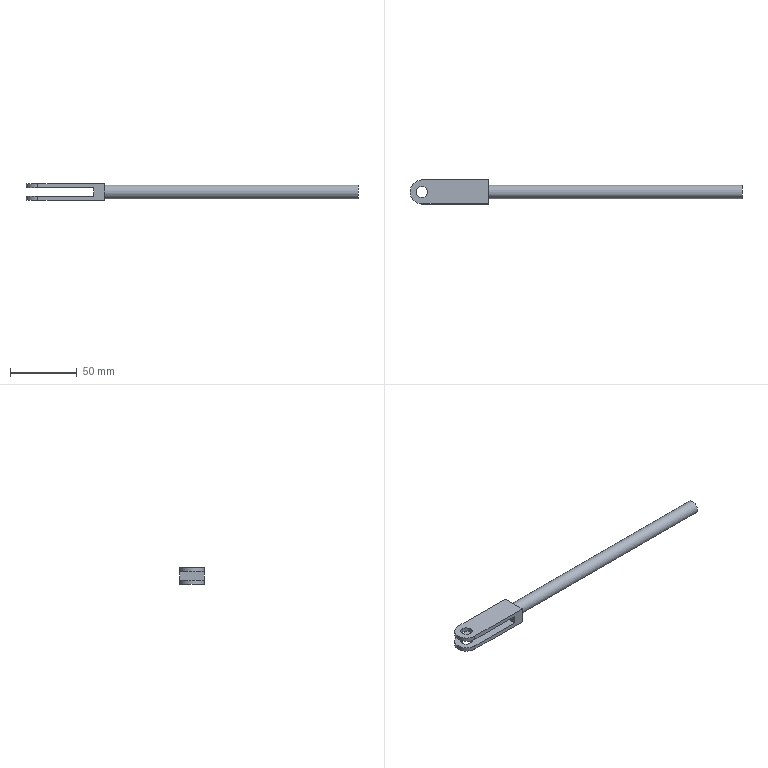Part | NX | features EXTRUDE 3, DATUM_CSYS 2, SKETCH 1, SWP104 1, UNITE 1 | 1 solid | 14 faces | box 249 x 18 x 12 mm | volume 21761 mm3 | plane 9 | cylinder 5 | commonest cylinder face diameters 8.5 x2 18 x2 10.051 x1
STEP:
#1=CARTESIAN_POINT('',(240.,0.,5.025));
#2=VERTEX_POINT('',#1);
#3=CARTESIAN_POINT('',(240.,0.,0.));
#4=DIRECTION('',(-1.,0.,0.));
#5=DIRECTION('',(0.,0.,1.));
#6=AXIS2_PLACEMENT_3D('',#3,#4,#5);
#7=CIRCLE('',#6,5.025);
#8=EDGE_CURVE('',#2,#2,#7,.T.);
#9=ORIENTED_EDGE('',*,*,#8,.F.);
#10=EDGE_LOOP('',(#9));
#11=FACE_BOUND('',#10,.T.);
#12=CARTESIAN_POINT('',(240.,0.,0.));
#13=DIRECTION('',(-1.,0.,0.));
#14=DIRECTION('',(0.,0.,1.));
#15=AXIS2_PLACEMENT_3D('',#12,#13,#14);
#16=PLANE('',#15);
#17=ADVANCED_FACE('',(#11),#16,.F.);
#18=ORIENTED_EDGE('',*,*,#8,.T.);
#19=EDGE_LOOP('',(#18));
#20=FACE_BOUND('',#19,.T.);
#21=CARTESIAN_POINT('',(50.,0.,5.025));
#22=VERTEX_POINT('',#21);
#23=CARTESIAN_POINT('',(50.,0.,0.));
#24=DIRECTION('',(-1.,0.,0.));
#25=DIRECTION('',(0.,0.,1.));
#26=AXIS2_PLACEMENT_3D('',#23,#24,#25);
#27=CIRCLE('',#26,5.025);
#28=EDGE_CURVE('',#22,#22,#27,.T.);
#29=ORIENTED_EDGE('',*,*,#28,.F.);
#30=EDGE_LOOP('',(#29));
#31=FACE_BOUND('',#30,.T.);
#32=CARTESIAN_POINT('',(50.,0.,0.));
#33=DIRECTION('',(-1.,0.,0.));
#34=DIRECTION('',(0.,0.,1.));
#35=AXIS2_PLACEMENT_3D('',#32,#33,#34);
#36=CYLINDRICAL_SURFACE('',#35,5.025);
#37=ADVANCED_FACE('',(#20,#31),#36,.T.);
#38=CARTESIAN_POINT('',(0.,9.,3.));
#39=VERTEX_POINT('',#38);
#40=CARTESIAN_POINT('',(0.,9.,6.));
#41=VERTEX_POINT('',#40);
#42=CARTESIAN_POINT('',(0.,9.,-6.));
#43=DIRECTION('',(0.,0.,1.));
#44=VECTOR('',#43,1000.);
#45=LINE('',#42,#44);
#46=EDGE_CURVE('',#39,#41,#45,.T.);
#47=ORIENTED_EDGE('',*,*,#46,.F.);
#48=CARTESIAN_POINT('',(0.,-9.,3.));
#49=VERTEX_POINT('',#48);
#50=CARTESIAN_POINT('',(0.,0.,3.));
#51=DIRECTION('',(0.,0.,1.));
#52=DIRECTION('',(-1.,0.,0.));
#53=AXIS2_PLACEMENT_3D('',#50,#51,#52);
#54=CIRCLE('',#53,9.);
#55=EDGE_CURVE('',#39,#49,#54,.T.);
#56=ORIENTED_EDGE('',*,*,#55,.T.);
#57=CARTESIAN_POINT('',(0.,-9.,6.));
#58=VERTEX_POINT('',#57);
#59=CARTESIAN_POINT('',(0.,-9.,-6.));
#60=DIRECTION('',(0.,0.,1.));
#61=VECTOR('',#60,1000.);
#62=LINE('',#59,#61);
#63=EDGE_CURVE('',#49,#58,#62,.T.);
#64=ORIENTED_EDGE('',*,*,#63,.T.);
#65=CARTESIAN_POINT('',(0.,0.,6.));
#66=DIRECTION('',(0.,0.,1.));
#67=DIRECTION('',(-1.,0.,0.));
#68=AXIS2_PLACEMENT_3D('',#65,#66,#67);
#69=CIRCLE('',#68,9.);
#70=EDGE_CURVE('',#41,#58,#69,.T.);
#71=ORIENTED_EDGE('',*,*,#70,.F.);
#72=EDGE_LOOP('',(#47,#56,#64,#71));
#73=FACE_BOUND('',#72,.T.);
#74=CARTESIAN_POINT('',(0.,0.,-6.));
#75=DIRECTION('',(0.,0.,1.));
#76=DIRECTION('',(1.,0.,0.));
#77=AXIS2_PLACEMENT_3D('',#74,#75,#76);
#78=CYLINDRICAL_SURFACE('',#77,9.);
#79=ADVANCED_FACE('',(#73),#78,.T.);
#80=CARTESIAN_POINT('',(42.,9.,-3.));
#81=VERTEX_POINT('',#80);
#82=CARTESIAN_POINT('',(0.,9.,-3.));
#83=VERTEX_POINT('',#82);
#84=CARTESIAN_POINT('',(42.,9.,-3.));
#85=DIRECTION('',(-1.,0.,0.));
#86=VECTOR('',#85,1000.);
#87=LINE('',#84,#86);
#88=EDGE_CURVE('',#81,#83,#87,.T.);
#89=ORIENTED_EDGE('',*,*,#88,.F.);
#90=CARTESIAN_POINT('',(42.,9.,3.));
#91=VERTEX_POINT('',#90);
#92=CARTESIAN_POINT('',(42.,9.,3.));
#93=DIRECTION('',(0.,0.,-1.));
#94=VECTOR('',#93,1000.);
#95=LINE('',#92,#94);
#96=EDGE_CURVE('',#91,#81,#95,.T.);
#97=ORIENTED_EDGE('',*,*,#96,.F.);
#98=CARTESIAN_POINT('',(42.,9.,3.));
#99=DIRECTION('',(-1.,0.,0.));
#100=VECTOR('',#99,1000.);
#101=LINE('',#98,#100);
#102=EDGE_CURVE('',#91,#39,#101,.T.);
#103=ORIENTED_EDGE('',*,*,#102,.T.);
#104=ORIENTED_EDGE('',*,*,#46,.T.);
#105=CARTESIAN_POINT('',(50.,9.,6.));
#106=VERTEX_POINT('',#105);
#107=CARTESIAN_POINT('',(50.,9.,6.));
#108=DIRECTION('',(-1.,0.,0.));
#109=VECTOR('',#108,1000.);
#110=LINE('',#107,#109);
#111=EDGE_CURVE('',#106,#41,#110,.T.);
#112=ORIENTED_EDGE('',*,*,#111,.F.);
#113=CARTESIAN_POINT('',(50.,9.,-6.));
#114=VERTEX_POINT('',#113);
#115=CARTESIAN_POINT('',(50.,9.,-6.));
#116=DIRECTION('',(0.,0.,1.));
#117=VECTOR('',#116,1000.);
#118=LINE('',#115,#117);
#119=EDGE_CURVE('',#114,#106,#118,.T.);
#120=ORIENTED_EDGE('',*,*,#119,.F.);
#121=CARTESIAN_POINT('',(0.,9.,-6.));
#122=VERTEX_POINT('',#121);
#123=CARTESIAN_POINT('',(50.,9.,-6.));
#124=DIRECTION('',(-1.,0.,0.));
#125=VECTOR('',#124,1000.);
#126=LINE('',#123,#125);
#127=EDGE_CURVE('',#114,#122,#126,.T.);
#128=ORIENTED_EDGE('',*,*,#127,.T.);
#129=CARTESIAN_POINT('',(0.,9.,-6.));
#130=DIRECTION('',(0.,0.,1.));
#131=VECTOR('',#130,1000.);
#132=LINE('',#129,#131);
#133=EDGE_CURVE('',#122,#83,#132,.T.);
#134=ORIENTED_EDGE('',*,*,#133,.T.);
#135=EDGE_LOOP('',(#89,#97,#103,#104,#112,#120,#128,#134));
#136=FACE_BOUND('',#135,.T.);
#137=CARTESIAN_POINT('',(50.,9.,-6.));
#138=DIRECTION('',(0.,1.,0.));
#139=DIRECTION('',(0.,0.,1.));
#140=AXIS2_PLACEMENT_3D('',#137,#138,#139);
#141=PLANE('',#140);
#142=ADVANCED_FACE('',(#136),#141,.T.);
#143=CARTESIAN_POINT('',(0.,-9.,-3.));
#144=VERTEX_POINT('',#143);
#145=CARTESIAN_POINT('',(0.,0.,-3.));
#146=DIRECTION('',(0.,0.,1.));
#147=DIRECTION('',(0.,1.,0.));
#148=AXIS2_PLACEMENT_3D('',#145,#146,#147);
#149=CIRCLE('',#148,9.);
#150=EDGE_CURVE('',#83,#144,#149,.T.);
#151=ORIENTED_EDGE('',*,*,#150,.F.);
#152=ORIENTED_EDGE('',*,*,#133,.F.);
#153=CARTESIAN_POINT('',(0.,-9.,-6.));
#154=VERTEX_POINT('',#153);
#155=CARTESIAN_POINT('',(0.,0.,-6.));
#156=DIRECTION('',(0.,0.,1.));
#157=DIRECTION('',(0.,1.,0.));
#158=AXIS2_PLACEMENT_3D('',#155,#156,#157);
#159=CIRCLE('',#158,9.);
#160=EDGE_CURVE('',#122,#154,#159,.T.);
#161=ORIENTED_EDGE('',*,*,#160,.T.);
#162=CARTESIAN_POINT('',(0.,-9.,-6.));
#163=DIRECTION('',(0.,0.,1.));
#164=VECTOR('',#163,1000.);
#165=LINE('',#162,#164);
#166=EDGE_CURVE('',#154,#144,#165,.T.);
#167=ORIENTED_EDGE('',*,*,#166,.T.);
#168=EDGE_LOOP('',(#151,#152,#161,#167));
#169=FACE_BOUND('',#168,.T.);
#170=CARTESIAN_POINT('',(0.,0.,-6.));
#171=DIRECTION('',(0.,0.,1.));
#172=DIRECTION('',(1.,0.,0.));
#173=AXIS2_PLACEMENT_3D('',#170,#171,#172);
#174=CYLINDRICAL_SURFACE('',#173,9.);
#175=ADVANCED_FACE('',(#169),#174,.T.);
#176=CARTESIAN_POINT('',(42.,-9.,-3.));
#177=VERTEX_POINT('',#176);
#178=CARTESIAN_POINT('',(0.,-9.,-3.));
#179=DIRECTION('',(1.,0.,0.));
#180=VECTOR('',#179,1000.);
#181=LINE('',#178,#180);
#182=EDGE_CURVE('',#144,#177,#181,.T.);
#183=ORIENTED_EDGE('',*,*,#182,.F.);
#184=ORIENTED_EDGE('',*,*,#166,.F.);
#185=CARTESIAN_POINT('',(50.,-9.,-6.));
#186=VERTEX_POINT('',#185);
#187=CARTESIAN_POINT('',(0.,-9.,-6.));
#188=DIRECTION('',(1.,0.,0.));
#189=VECTOR('',#188,1000.);
#190=LINE('',#187,#189);
#191=EDGE_CURVE('',#154,#186,#190,.T.);
#192=ORIENTED_EDGE('',*,*,#191,.T.);
#193=CARTESIAN_POINT('',(50.,-9.,6.));
#194=VERTEX_POINT('',#193);
#195=CARTESIAN_POINT('',(50.,-9.,-6.));
#196=DIRECTION('',(0.,0.,1.));
#197=VECTOR('',#196,1000.);
#198=LINE('',#195,#197);
#199=EDGE_CURVE('',#186,#194,#198,.T.);
#200=ORIENTED_EDGE('',*,*,#199,.T.);
#201=CARTESIAN_POINT('',(0.,-9.,6.));
#202=DIRECTION('',(1.,0.,0.));
#203=VECTOR('',#202,1000.);
#204=LINE('',#201,#203);
#205=EDGE_CURVE('',#58,#194,#204,.T.);
#206=ORIENTED_EDGE('',*,*,#205,.F.);
#207=ORIENTED_EDGE('',*,*,#63,.F.);
#208=CARTESIAN_POINT('',(42.,-9.,3.));
#209=VERTEX_POINT('',#208);
#210=CARTESIAN_POINT('',(0.,-9.,3.));
#211=DIRECTION('',(1.,0.,0.));
#212=VECTOR('',#211,1000.);
#213=LINE('',#210,#212);
#214=EDGE_CURVE('',#49,#209,#213,.T.);
#215=ORIENTED_EDGE('',*,*,#214,.T.);
#216=CARTESIAN_POINT('',(42.,-9.,3.));
#217=DIRECTION('',(0.,0.,-1.));
#218=VECTOR('',#217,1000.);
#219=LINE('',#216,#218);
#220=EDGE_CURVE('',#209,#177,#219,.T.);
#221=ORIENTED_EDGE('',*,*,#220,.T.);
#222=EDGE_LOOP('',(#183,#184,#192,#200,#206,#207,#215,#221));
#223=FACE_BOUND('',#222,.T.);
#224=CARTESIAN_POINT('',(0.,-9.,-6.));
#225=DIRECTION('',(0.,-1.,0.));
#226=DIRECTION('',(0.,0.,-1.));
#227=AXIS2_PLACEMENT_3D('',#224,#225,#226);
#228=PLANE('',#227);
#229=ADVANCED_FACE('',(#223),#228,.T.);
#230=ORIENTED_EDGE('',*,*,#28,.T.);
#231=EDGE_LOOP('',(#230));
#232=FACE_BOUND('',#231,.T.);
#233=CARTESIAN_POINT('',(50.,-9.,6.));
#234=DIRECTION('',(0.,1.,0.));
#235=VECTOR('',#234,1000.);
#236=LINE('',#233,#235);
#237=EDGE_CURVE('',#194,#106,#236,.T.);
#238=ORIENTED_EDGE('',*,*,#237,.F.);
#239=ORIENTED_EDGE('',*,*,#199,.F.);
#240=CARTESIAN_POINT('',(50.,-9.,-6.));
#241=DIRECTION('',(0.,1.,0.));
#242=VECTOR('',#241,1000.);
#243=LINE('',#240,#242);
#244=EDGE_CURVE('',#186,#114,#243,.T.);
#245=ORIENTED_EDGE('',*,*,#244,.T.);
#246=ORIENTED_EDGE('',*,*,#119,.T.);
#247=EDGE_LOOP('',(#238,#239,#245,#246));
#248=FACE_BOUND('',#247,.T.);
#249=CARTESIAN_POINT('',(50.,-9.,-6.));
#250=DIRECTION('',(1.,0.,0.));
#251=DIRECTION('',(0.,0.,-1.));
#252=AXIS2_PLACEMENT_3D('',#249,#250,#251);
#253=PLANE('',#252);
#254=ADVANCED_FACE('',(#232,#248),#253,.T.);
#255=CARTESIAN_POINT('',(4.25,0.,-6.));
#256=VERTEX_POINT('',#255);
#257=CARTESIAN_POINT('',(0.,0.,-6.));
#258=DIRECTION('',(0.,0.,1.));
#259=DIRECTION('',(1.,0.,0.));
#260=AXIS2_PLACEMENT_3D('',#257,#258,#259);
#261=CIRCLE('',#260,4.25);
#262=EDGE_CURVE('',#256,#256,#261,.F.);
#263=ORIENTED_EDGE('',*,*,#262,.F.);
#264=EDGE_LOOP('',(#263));
#265=FACE_BOUND('',#264,.T.);
#266=ORIENTED_EDGE('',*,*,#127,.F.);
#267=ORIENTED_EDGE('',*,*,#244,.F.);
#268=ORIENTED_EDGE('',*,*,#191,.F.);
#269=ORIENTED_EDGE('',*,*,#160,.F.);
#270=EDGE_LOOP('',(#266,#267,#268,#269));
#271=FACE_BOUND('',#270,.T.);
#272=CARTESIAN_POINT('',(0.,0.,-6.));
#273=DIRECTION('',(0.,0.,1.));
#274=DIRECTION('',(1.,0.,0.));
#275=AXIS2_PLACEMENT_3D('',#272,#273,#274);
#276=PLANE('',#275);
#277=ADVANCED_FACE('',(#265,#271),#276,.F.);
#278=CARTESIAN_POINT('',(4.25,0.,6.));
#279=VERTEX_POINT('',#278);
#280=CARTESIAN_POINT('',(0.,0.,6.));
#281=DIRECTION('',(0.,0.,1.));
#282=DIRECTION('',(1.,0.,0.));
#283=AXIS2_PLACEMENT_3D('',#280,#281,#282);
#284=CIRCLE('',#283,4.25);
#285=EDGE_CURVE('',#279,#279,#284,.F.);
#286=ORIENTED_EDGE('',*,*,#285,.T.);
#287=EDGE_LOOP('',(#286));
#288=FACE_BOUND('',#287,.T.);
#289=ORIENTED_EDGE('',*,*,#111,.T.);
#290=ORIENTED_EDGE('',*,*,#70,.T.);
#291=ORIENTED_EDGE('',*,*,#205,.T.);
#292=ORIENTED_EDGE('',*,*,#237,.T.);
#293=EDGE_LOOP('',(#289,#290,#291,#292));
#294=FACE_BOUND('',#293,.T.);
#295=CARTESIAN_POINT('',(0.,0.,6.));
#296=DIRECTION('',(0.,0.,1.));
#297=DIRECTION('',(1.,0.,0.));
#298=AXIS2_PLACEMENT_3D('',#295,#296,#297);
#299=PLANE('',#298);
#300=ADVANCED_FACE('',(#288,#294),#299,.T.);
#301=CARTESIAN_POINT('',(42.,-9.,-3.));
#302=DIRECTION('',(0.,1.,0.));
#303=VECTOR('',#302,1000.);
#304=LINE('',#301,#303);
#305=EDGE_CURVE('',#81,#177,#304,.F.);
#306=ORIENTED_EDGE('',*,*,#305,.T.);
#307=ORIENTED_EDGE('',*,*,#220,.F.);
#308=CARTESIAN_POINT('',(42.,-9.,3.));
#309=DIRECTION('',(0.,1.,0.));
#310=VECTOR('',#309,1000.);
#311=LINE('',#308,#310);
#312=EDGE_CURVE('',#91,#209,#311,.F.);
#313=ORIENTED_EDGE('',*,*,#312,.F.);
#314=ORIENTED_EDGE('',*,*,#96,.T.);
#315=EDGE_LOOP('',(#306,#307,#313,#314));
#316=FACE_BOUND('',#315,.T.);
#317=CARTESIAN_POINT('',(42.,-9.,3.));
#318=DIRECTION('',(-1.,0.,0.));
#319=DIRECTION('',(0.,0.,1.));
#320=AXIS2_PLACEMENT_3D('',#317,#318,#319);
#321=PLANE('',#320);
#322=ADVANCED_FACE('',(#316),#321,.T.);
#323=CARTESIAN_POINT('',(4.25,0.,3.));
#324=VERTEX_POINT('',#323);
#325=CARTESIAN_POINT('',(0.,0.,3.));
#326=DIRECTION('',(0.,0.,1.));
#327=DIRECTION('',(1.,0.,0.));
#328=AXIS2_PLACEMENT_3D('',#325,#326,#327);
#329=CIRCLE('',#328,4.25);
#330=EDGE_CURVE('',#324,#324,#329,.F.);
#331=ORIENTED_EDGE('',*,*,#330,.F.);
#332=EDGE_LOOP('',(#331));
#333=FACE_BOUND('',#332,.T.);
#334=ORIENTED_EDGE('',*,*,#55,.F.);
#335=ORIENTED_EDGE('',*,*,#102,.F.);
#336=ORIENTED_EDGE('',*,*,#312,.T.);
#337=ORIENTED_EDGE('',*,*,#214,.F.);
#338=EDGE_LOOP('',(#334,#335,#336,#337));
#339=FACE_BOUND('',#338,.T.);
#340=CARTESIAN_POINT('',(0.,0.,3.));
#341=DIRECTION('',(0.,0.,1.));
#342=DIRECTION('',(1.,0.,0.));
#343=AXIS2_PLACEMENT_3D('',#340,#341,#342);
#344=PLANE('',#343);
#345=ADVANCED_FACE('',(#333,#339),#344,.F.);
#346=CARTESIAN_POINT('',(4.25,0.,-3.));
#347=VERTEX_POINT('',#346);
#348=CARTESIAN_POINT('',(0.,0.,-3.));
#349=DIRECTION('',(0.,0.,1.));
#350=DIRECTION('',(1.,0.,0.));
#351=AXIS2_PLACEMENT_3D('',#348,#349,#350);
#352=CIRCLE('',#351,4.25);
#353=EDGE_CURVE('',#347,#347,#352,.F.);
#354=ORIENTED_EDGE('',*,*,#353,.T.);
#355=EDGE_LOOP('',(#354));
#356=FACE_BOUND('',#355,.T.);
#357=ORIENTED_EDGE('',*,*,#182,.T.);
#358=ORIENTED_EDGE('',*,*,#305,.F.);
#359=ORIENTED_EDGE('',*,*,#88,.T.);
#360=ORIENTED_EDGE('',*,*,#150,.T.);
#361=EDGE_LOOP('',(#357,#358,#359,#360));
#362=FACE_BOUND('',#361,.T.);
#363=CARTESIAN_POINT('',(0.,0.,-3.));
#364=DIRECTION('',(0.,0.,1.));
#365=DIRECTION('',(1.,0.,0.));
#366=AXIS2_PLACEMENT_3D('',#363,#364,#365);
#367=PLANE('',#366);
#368=ADVANCED_FACE('',(#356,#362),#367,.T.);
#369=ORIENTED_EDGE('',*,*,#353,.F.);
#370=EDGE_LOOP('',(#369));
#371=FACE_BOUND('',#370,.T.);
#372=ORIENTED_EDGE('',*,*,#262,.T.);
#373=EDGE_LOOP('',(#372));
#374=FACE_BOUND('',#373,.T.);
#375=CARTESIAN_POINT('',(0.,0.,10.5));
#376=DIRECTION('',(0.,0.,-1.));
#377=DIRECTION('',(-1.,0.,0.));
#378=AXIS2_PLACEMENT_3D('',#375,#376,#377);
#379=CYLINDRICAL_SURFACE('',#378,4.25);
#380=ADVANCED_FACE('',(#371,#374),#379,.F.);
#381=ORIENTED_EDGE('',*,*,#285,.F.);
#382=EDGE_LOOP('',(#381));
#383=FACE_BOUND('',#382,.T.);
#384=ORIENTED_EDGE('',*,*,#330,.T.);
#385=EDGE_LOOP('',(#384));
#386=FACE_BOUND('',#385,.T.);
#387=CARTESIAN_POINT('',(0.,0.,10.5));
#388=DIRECTION('',(0.,0.,-1.));
#389=DIRECTION('',(-1.,0.,0.));
#390=AXIS2_PLACEMENT_3D('',#387,#388,#389);
#391=CYLINDRICAL_SURFACE('',#390,4.25);
#392=ADVANCED_FACE('',(#383,#386),#391,.F.);
#393=CLOSED_SHELL('',(#17,#37,#79,#142,#175,#229,#254,#277,#300,#322,#345,#368,#380,#392));
#394=MANIFOLD_SOLID_BREP('',#393);
#395=(LENGTH_UNIT()NAMED_UNIT(*)SI_UNIT(.MILLI.,.METRE.));
#396=UNCERTAINTY_MEASURE_WITH_UNIT(LENGTH_MEASURE(0.00001),#395,'','');
#397=(NAMED_UNIT(*)PLANE_ANGLE_UNIT()SI_UNIT($,.RADIAN.));
#398=(NAMED_UNIT(*)SI_UNIT($,.STERADIAN.)SOLID_ANGLE_UNIT());
#399=(GEOMETRIC_REPRESENTATION_CONTEXT(3)GLOBAL_UNCERTAINTY_ASSIGNED_CONTEXT((#396))GLOBAL_UNIT_ASSIGNED_CONTEXT((#395,#397,#398))REPRESENTATION_CONTEXT('',''));
#400=ADVANCED_BREP_SHAPE_REPRESENTATION('',(#394),#399);